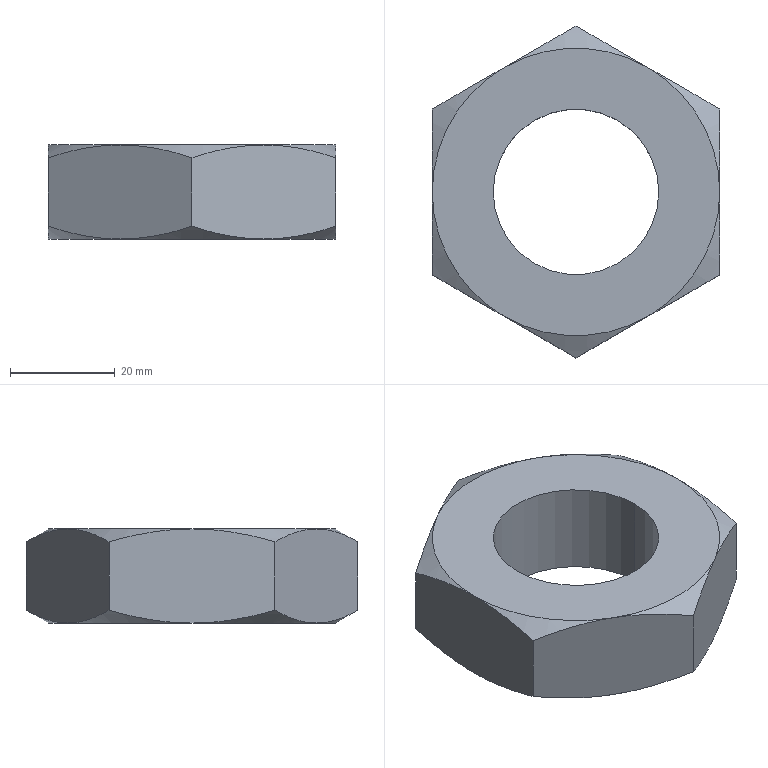Part | SolidWorks | features BaseBody 1 | 1 solid | 22 faces | box 55 x 63.509 x 18 mm | volume 32614 mm3 | cone 12 | plane 8 | cylinder 2 | commonest cylinder face diameters 31.67 x2
STEP:
#1=CARTESIAN_POINT('',(15.835,0.,18.));
#2=VERTEX_POINT('',#1);
#3=CARTESIAN_POINT('',(-15.835,0.,18.));
#4=VERTEX_POINT('',#3);
#5=CARTESIAN_POINT('',(0.,0.,18.));
#6=DIRECTION('',(0.,0.,-1.));
#7=DIRECTION('',(-1.,0.,0.));
#8=AXIS2_PLACEMENT_3D('',#5,#6,#7);
#9=CIRCLE('',#8,15.835);
#10=EDGE_CURVE('',#2,#4,#9,.T.);
#11=ORIENTED_EDGE('',*,*,#10,.F.);
#12=CARTESIAN_POINT('',(15.835,0.,0.));
#13=VERTEX_POINT('',#12);
#14=CARTESIAN_POINT('',(15.835,0.,18.));
#15=DIRECTION('',(0.,0.,-1.));
#16=VECTOR('',#15,1000.);
#17=LINE('',#14,#16);
#18=EDGE_CURVE('',#2,#13,#17,.T.);
#19=ORIENTED_EDGE('',*,*,#18,.T.);
#20=CARTESIAN_POINT('',(-15.835,0.,0.));
#21=VERTEX_POINT('',#20);
#22=CARTESIAN_POINT('',(0.,0.,0.));
#23=DIRECTION('',(0.,0.,-1.));
#24=DIRECTION('',(-1.,0.,0.));
#25=AXIS2_PLACEMENT_3D('',#22,#23,#24);
#26=CIRCLE('',#25,15.835);
#27=EDGE_CURVE('',#13,#21,#26,.T.);
#28=ORIENTED_EDGE('',*,*,#27,.T.);
#29=CARTESIAN_POINT('',(-15.835,0.,18.));
#30=DIRECTION('',(0.,0.,-1.));
#31=VECTOR('',#30,1000.);
#32=LINE('',#29,#31);
#33=EDGE_CURVE('',#4,#21,#32,.T.);
#34=ORIENTED_EDGE('',*,*,#33,.F.);
#35=EDGE_LOOP('',(#11,#19,#28,#34));
#36=FACE_OUTER_BOUND('',#35,.T.);
#37=CARTESIAN_POINT('',(0.,0.,18.));
#38=DIRECTION('',(0.,0.,-1.));
#39=DIRECTION('',(-1.,0.,0.));
#40=AXIS2_PLACEMENT_3D('',#37,#38,#39);
#41=CYLINDRICAL_SURFACE('',#40,15.835);
#42=ADVANCED_FACE('',(#36),#41,.F.);
#43=CARTESIAN_POINT('',(13.75,-23.816,0.));
#44=VERTEX_POINT('',#43);
#45=CARTESIAN_POINT('',(27.5,0.,0.));
#46=VERTEX_POINT('',#45);
#47=CARTESIAN_POINT('',(0.,0.,0.));
#48=DIRECTION('',(0.,0.,1.));
#49=DIRECTION('',(1.,0.,0.));
#50=AXIS2_PLACEMENT_3D('',#47,#48,#49);
#51=CIRCLE('',#50,27.5);
#52=EDGE_CURVE('',#44,#46,#51,.T.);
#53=ORIENTED_EDGE('',*,*,#52,.F.);
#54=CARTESIAN_POINT('',(-13.75,-23.816,0.));
#55=VERTEX_POINT('',#54);
#56=CARTESIAN_POINT('',(0.,0.,0.));
#57=DIRECTION('',(0.,0.,1.));
#58=DIRECTION('',(1.,0.,0.));
#59=AXIS2_PLACEMENT_3D('',#56,#57,#58);
#60=CIRCLE('',#59,27.5);
#61=EDGE_CURVE('',#55,#44,#60,.T.);
#62=ORIENTED_EDGE('',*,*,#61,.F.);
#63=CARTESIAN_POINT('',(-27.5,0.,0.));
#64=VERTEX_POINT('',#63);
#65=CARTESIAN_POINT('',(0.,0.,0.));
#66=DIRECTION('',(0.,0.,1.));
#67=DIRECTION('',(1.,0.,0.));
#68=AXIS2_PLACEMENT_3D('',#65,#66,#67);
#69=CIRCLE('',#68,27.5);
#70=EDGE_CURVE('',#64,#55,#69,.T.);
#71=ORIENTED_EDGE('',*,*,#70,.F.);
#72=CARTESIAN_POINT('',(-13.75,23.816,0.));
#73=VERTEX_POINT('',#72);
#74=CARTESIAN_POINT('',(0.,0.,0.));
#75=DIRECTION('',(0.,0.,1.));
#76=DIRECTION('',(0.,-1.,0.));
#77=AXIS2_PLACEMENT_3D('',#74,#75,#76);
#78=CIRCLE('',#77,27.5);
#79=EDGE_CURVE('',#73,#64,#78,.T.);
#80=ORIENTED_EDGE('',*,*,#79,.F.);
#81=CARTESIAN_POINT('',(13.75,23.816,0.));
#82=VERTEX_POINT('',#81);
#83=CARTESIAN_POINT('',(0.,0.,0.));
#84=DIRECTION('',(0.,0.,1.));
#85=DIRECTION('',(1.,0.,0.));
#86=AXIS2_PLACEMENT_3D('',#83,#84,#85);
#87=CIRCLE('',#86,27.5);
#88=EDGE_CURVE('',#82,#73,#87,.T.);
#89=ORIENTED_EDGE('',*,*,#88,.F.);
#90=CARTESIAN_POINT('',(0.,0.,0.));
#91=DIRECTION('',(0.,0.,1.));
#92=DIRECTION('',(1.,0.,0.));
#93=AXIS2_PLACEMENT_3D('',#90,#91,#92);
#94=CIRCLE('',#93,27.5);
#95=EDGE_CURVE('',#46,#82,#94,.T.);
#96=ORIENTED_EDGE('',*,*,#95,.F.);
#97=EDGE_LOOP('',(#53,#62,#71,#80,#89,#96));
#98=FACE_OUTER_BOUND('',#97,.T.);
#99=CARTESIAN_POINT('',(0.,0.,0.));
#100=DIRECTION('',(0.,0.,-1.));
#101=DIRECTION('',(-1.,0.,0.));
#102=AXIS2_PLACEMENT_3D('',#99,#100,#101);
#103=CIRCLE('',#102,15.835);
#104=EDGE_CURVE('',#21,#13,#103,.T.);
#105=ORIENTED_EDGE('',*,*,#104,.F.);
#106=ORIENTED_EDGE('',*,*,#27,.F.);
#107=EDGE_LOOP('',(#105,#106));
#108=FACE_BOUND('',#107,.T.);
#109=CARTESIAN_POINT('',(-27.5,47.631,0.));
#110=DIRECTION('',(0.,0.,1.));
#111=DIRECTION('',(1.,0.,0.));
#112=AXIS2_PLACEMENT_3D('',#109,#110,#111);
#113=PLANE('',#112);
#114=ADVANCED_FACE('',(#98,#108),#113,.F.);
#115=CARTESIAN_POINT('',(27.5,15.877,2.456));
#116=VERTEX_POINT('',#115);
#117=CARTESIAN_POINT('',(27.5,15.877,2.456));
#118=CARTESIAN_POINT('',(27.5,13.283,1.707));
#119=CARTESIAN_POINT('',(27.5,10.669,1.09));
#120=CARTESIAN_POINT('',(27.5,5.383,0.2348));
#121=CARTESIAN_POINT('',(27.5,2.71,0.));
#122=CARTESIAN_POINT('',(27.5,0.,0.));
#123=B_SPLINE_CURVE_WITH_KNOTS('',3,(#117,#118,#119,#120,#121,#122),.UNSPECIFIED.,.F.,.F.,(4,2,4),(0.,0.008033,0.01607),.UNSPECIFIED.);
#124=EDGE_CURVE('',#116,#46,#123,.T.);
#125=ORIENTED_EDGE('',*,*,#124,.T.);
#126=ORIENTED_EDGE('',*,*,#95,.T.);
#127=CARTESIAN_POINT('',(13.75,23.816,0.));
#128=CARTESIAN_POINT('',(16.097,22.461,0.));
#129=CARTESIAN_POINT('',(18.412,21.124,0.2348));
#130=CARTESIAN_POINT('',(22.99,18.481,1.09));
#131=CARTESIAN_POINT('',(25.254,17.174,1.707));
#132=CARTESIAN_POINT('',(27.5,15.877,2.456));
#133=B_SPLINE_CURVE_WITH_KNOTS('',3,(#127,#128,#129,#130,#131,#132),.UNSPECIFIED.,.F.,.F.,(4,2,4),(0.,0.008033,0.01607),.UNSPECIFIED.);
#134=EDGE_CURVE('',#82,#116,#133,.T.);
#135=ORIENTED_EDGE('',*,*,#134,.T.);
#136=EDGE_LOOP('',(#125,#126,#135));
#137=FACE_OUTER_BOUND('',#136,.T.);
#138=CARTESIAN_POINT('',(0.,0.,2.471));
#139=DIRECTION('',(0.,0.,1.));
#140=DIRECTION('',(1.,0.,0.));
#141=AXIS2_PLACEMENT_3D('',#138,#139,#140);
#142=CONICAL_SURFACE('',#141,31.78,1.047);
#143=ADVANCED_FACE('',(#137),#142,.T.);
#144=ORIENTED_EDGE('',*,*,#52,.T.);
#145=CARTESIAN_POINT('',(27.5,-15.877,2.456));
#146=VERTEX_POINT('',#145);
#147=CARTESIAN_POINT('',(27.5,0.,0.));
#148=CARTESIAN_POINT('',(27.5,-2.71,0.));
#149=CARTESIAN_POINT('',(27.5,-5.383,0.2348));
#150=CARTESIAN_POINT('',(27.5,-10.669,1.09));
#151=CARTESIAN_POINT('',(27.5,-13.283,1.707));
#152=CARTESIAN_POINT('',(27.5,-15.877,2.456));
#153=B_SPLINE_CURVE_WITH_KNOTS('',3,(#147,#148,#149,#150,#151,#152),.UNSPECIFIED.,.F.,.F.,(4,2,4),(0.,0.008033,0.01607),.UNSPECIFIED.);
#154=EDGE_CURVE('',#46,#146,#153,.T.);
#155=ORIENTED_EDGE('',*,*,#154,.T.);
#156=CARTESIAN_POINT('',(27.5,-15.877,2.456));
#157=CARTESIAN_POINT('',(25.254,-17.174,1.707));
#158=CARTESIAN_POINT('',(22.99,-18.481,1.09));
#159=CARTESIAN_POINT('',(18.412,-21.124,0.2348));
#160=CARTESIAN_POINT('',(16.097,-22.461,0.));
#161=CARTESIAN_POINT('',(13.75,-23.816,0.));
#162=B_SPLINE_CURVE_WITH_KNOTS('',3,(#156,#157,#158,#159,#160,#161),.UNSPECIFIED.,.F.,.F.,(4,2,4),(0.,0.008033,0.01607),.UNSPECIFIED.);
#163=EDGE_CURVE('',#146,#44,#162,.T.);
#164=ORIENTED_EDGE('',*,*,#163,.T.);
#165=EDGE_LOOP('',(#144,#155,#164));
#166=FACE_OUTER_BOUND('',#165,.T.);
#167=CARTESIAN_POINT('',(0.,0.,2.471));
#168=DIRECTION('',(0.,0.,1.));
#169=DIRECTION('',(1.,0.,0.));
#170=AXIS2_PLACEMENT_3D('',#167,#168,#169);
#171=CONICAL_SURFACE('',#170,31.78,1.047);
#172=ADVANCED_FACE('',(#166),#171,.T.);
#173=ORIENTED_EDGE('',*,*,#61,.T.);
#174=CARTESIAN_POINT('',(-0.000000014,-31.754,2.456));
#175=VERTEX_POINT('',#174);
#176=CARTESIAN_POINT('',(13.75,-23.816,0.));
#177=CARTESIAN_POINT('',(11.403,-25.17,0.));
#178=CARTESIAN_POINT('',(9.088,-26.507,0.2348));
#179=CARTESIAN_POINT('',(4.51,-29.15,1.09));
#180=CARTESIAN_POINT('',(2.246,-30.457,1.707));
#181=CARTESIAN_POINT('',(-0.000000014,-31.754,2.456));
#182=B_SPLINE_CURVE_WITH_KNOTS('',3,(#176,#177,#178,#179,#180,#181),.UNSPECIFIED.,.F.,.F.,(4,2,4),(0.,0.008033,0.01607),.UNSPECIFIED.);
#183=EDGE_CURVE('',#44,#175,#182,.T.);
#184=ORIENTED_EDGE('',*,*,#183,.T.);
#185=CARTESIAN_POINT('',(-0.000000014,-31.754,2.456));
#186=CARTESIAN_POINT('',(-2.246,-30.457,1.707));
#187=CARTESIAN_POINT('',(-4.51,-29.15,1.09));
#188=CARTESIAN_POINT('',(-9.088,-26.507,0.2348));
#189=CARTESIAN_POINT('',(-11.403,-25.17,0.));
#190=CARTESIAN_POINT('',(-13.75,-23.816,0.));
#191=B_SPLINE_CURVE_WITH_KNOTS('',3,(#185,#186,#187,#188,#189,#190),.UNSPECIFIED.,.F.,.F.,(4,2,4),(0.,0.008033,0.01607),.UNSPECIFIED.);
#192=EDGE_CURVE('',#175,#55,#191,.T.);
#193=ORIENTED_EDGE('',*,*,#192,.T.);
#194=EDGE_LOOP('',(#173,#184,#193));
#195=FACE_OUTER_BOUND('',#194,.T.);
#196=CARTESIAN_POINT('',(0.,0.,2.471));
#197=DIRECTION('',(0.,0.,1.));
#198=DIRECTION('',(1.,0.,0.));
#199=AXIS2_PLACEMENT_3D('',#196,#197,#198);
#200=CONICAL_SURFACE('',#199,31.78,1.047);
#201=ADVANCED_FACE('',(#195),#200,.T.);
#202=ORIENTED_EDGE('',*,*,#70,.T.);
#203=CARTESIAN_POINT('',(-27.5,-15.877,2.456));
#204=VERTEX_POINT('',#203);
#205=CARTESIAN_POINT('',(-13.75,-23.816,0.));
#206=CARTESIAN_POINT('',(-16.097,-22.461,0.));
#207=CARTESIAN_POINT('',(-18.412,-21.124,0.2348));
#208=CARTESIAN_POINT('',(-22.99,-18.481,1.09));
#209=CARTESIAN_POINT('',(-25.254,-17.174,1.707));
#210=CARTESIAN_POINT('',(-27.5,-15.877,2.456));
#211=B_SPLINE_CURVE_WITH_KNOTS('',3,(#205,#206,#207,#208,#209,#210),.UNSPECIFIED.,.F.,.F.,(4,2,4),(0.,0.008033,0.01607),.UNSPECIFIED.);
#212=EDGE_CURVE('',#55,#204,#211,.T.);
#213=ORIENTED_EDGE('',*,*,#212,.T.);
#214=CARTESIAN_POINT('',(-27.5,-15.877,2.456));
#215=CARTESIAN_POINT('',(-27.5,-13.283,1.707));
#216=CARTESIAN_POINT('',(-27.5,-10.669,1.09));
#217=CARTESIAN_POINT('',(-27.5,-5.383,0.2348));
#218=CARTESIAN_POINT('',(-27.5,-2.71,0.));
#219=CARTESIAN_POINT('',(-27.5,0.,0.));
#220=B_SPLINE_CURVE_WITH_KNOTS('',3,(#214,#215,#216,#217,#218,#219),.UNSPECIFIED.,.F.,.F.,(4,2,4),(0.,0.008033,0.01607),.UNSPECIFIED.);
#221=EDGE_CURVE('',#204,#64,#220,.T.);
#222=ORIENTED_EDGE('',*,*,#221,.T.);
#223=EDGE_LOOP('',(#202,#213,#222));
#224=FACE_OUTER_BOUND('',#223,.T.);
#225=CARTESIAN_POINT('',(0.,0.,2.471));
#226=DIRECTION('',(0.,0.,1.));
#227=DIRECTION('',(1.,0.,0.));
#228=AXIS2_PLACEMENT_3D('',#225,#226,#227);
#229=CONICAL_SURFACE('',#228,31.78,1.047);
#230=ADVANCED_FACE('',(#224),#229,.T.);
#231=CARTESIAN_POINT('',(-27.5,15.877,2.456));
#232=VERTEX_POINT('',#231);
#233=CARTESIAN_POINT('',(-27.5,15.877,2.456));
#234=CARTESIAN_POINT('',(-25.254,17.174,1.707));
#235=CARTESIAN_POINT('',(-22.99,18.481,1.09));
#236=CARTESIAN_POINT('',(-18.412,21.124,0.2348));
#237=CARTESIAN_POINT('',(-16.097,22.461,0.));
#238=CARTESIAN_POINT('',(-13.75,23.816,0.));
#239=B_SPLINE_CURVE_WITH_KNOTS('',3,(#233,#234,#235,#236,#237,#238),.UNSPECIFIED.,.F.,.F.,(4,2,4),(0.,0.008033,0.01607),.UNSPECIFIED.);
#240=EDGE_CURVE('',#232,#73,#239,.T.);
#241=ORIENTED_EDGE('',*,*,#240,.T.);
#242=ORIENTED_EDGE('',*,*,#79,.T.);
#243=CARTESIAN_POINT('',(-27.5,0.,0.));
#244=CARTESIAN_POINT('',(-27.5,2.71,0.));
#245=CARTESIAN_POINT('',(-27.5,5.383,0.2348));
#246=CARTESIAN_POINT('',(-27.5,10.669,1.09));
#247=CARTESIAN_POINT('',(-27.5,13.283,1.707));
#248=CARTESIAN_POINT('',(-27.5,15.877,2.456));
#249=B_SPLINE_CURVE_WITH_KNOTS('',3,(#243,#244,#245,#246,#247,#248),.UNSPECIFIED.,.F.,.F.,(4,2,4),(0.,0.008033,0.01607),.UNSPECIFIED.);
#250=EDGE_CURVE('',#64,#232,#249,.T.);
#251=ORIENTED_EDGE('',*,*,#250,.T.);
#252=EDGE_LOOP('',(#241,#242,#251));
#253=FACE_OUTER_BOUND('',#252,.T.);
#254=CARTESIAN_POINT('',(0.,0.,2.471));
#255=DIRECTION('',(0.,0.,1.));
#256=DIRECTION('',(0.,-1.,0.));
#257=AXIS2_PLACEMENT_3D('',#254,#255,#256);
#258=CONICAL_SURFACE('',#257,31.78,1.047);
#259=ADVANCED_FACE('',(#253),#258,.T.);
#260=CARTESIAN_POINT('',(-0.000000038,31.754,2.456));
#261=VERTEX_POINT('',#260);
#262=CARTESIAN_POINT('',(-0.000000038,31.754,2.456));
#263=CARTESIAN_POINT('',(2.246,30.457,1.707));
#264=CARTESIAN_POINT('',(4.51,29.15,1.09));
#265=CARTESIAN_POINT('',(9.088,26.507,0.2348));
#266=CARTESIAN_POINT('',(11.403,25.17,0.));
#267=CARTESIAN_POINT('',(13.75,23.816,0.));
#268=B_SPLINE_CURVE_WITH_KNOTS('',3,(#262,#263,#264,#265,#266,#267),.UNSPECIFIED.,.F.,.F.,(4,2,4),(0.,0.008033,0.01607),.UNSPECIFIED.);
#269=EDGE_CURVE('',#261,#82,#268,.T.);
#270=ORIENTED_EDGE('',*,*,#269,.T.);
#271=ORIENTED_EDGE('',*,*,#88,.T.);
#272=CARTESIAN_POINT('',(-13.75,23.816,0.));
#273=CARTESIAN_POINT('',(-11.403,25.17,0.));
#274=CARTESIAN_POINT('',(-9.088,26.507,0.2348));
#275=CARTESIAN_POINT('',(-4.51,29.15,1.09));
#276=CARTESIAN_POINT('',(-2.246,30.457,1.707));
#277=CARTESIAN_POINT('',(-0.000000038,31.754,2.456));
#278=B_SPLINE_CURVE_WITH_KNOTS('',3,(#272,#273,#274,#275,#276,#277),.UNSPECIFIED.,.F.,.F.,(4,2,4),(0.,0.008033,0.01607),.UNSPECIFIED.);
#279=EDGE_CURVE('',#73,#261,#278,.T.);
#280=ORIENTED_EDGE('',*,*,#279,.T.);
#281=EDGE_LOOP('',(#270,#271,#280));
#282=FACE_OUTER_BOUND('',#281,.T.);
#283=CARTESIAN_POINT('',(0.,0.,2.471));
#284=DIRECTION('',(0.,0.,1.));
#285=DIRECTION('',(1.,0.,0.));
#286=AXIS2_PLACEMENT_3D('',#283,#284,#285);
#287=CONICAL_SURFACE('',#286,31.78,1.047);
#288=ADVANCED_FACE('',(#282),#287,.T.);
#289=ORIENTED_EDGE('',*,*,#18,.F.);
#290=CARTESIAN_POINT('',(0.,0.,18.));
#291=DIRECTION('',(0.,0.,-1.));
#292=DIRECTION('',(-1.,0.,0.));
#293=AXIS2_PLACEMENT_3D('',#290,#291,#292);
#294=CIRCLE('',#293,15.835);
#295=EDGE_CURVE('',#4,#2,#294,.T.);
#296=ORIENTED_EDGE('',*,*,#295,.F.);
#297=ORIENTED_EDGE('',*,*,#33,.T.);
#298=ORIENTED_EDGE('',*,*,#104,.T.);
#299=EDGE_LOOP('',(#289,#296,#297,#298));
#300=FACE_OUTER_BOUND('',#299,.T.);
#301=CARTESIAN_POINT('',(0.,0.,18.));
#302=DIRECTION('',(0.,0.,-1.));
#303=DIRECTION('',(-1.,0.,0.));
#304=AXIS2_PLACEMENT_3D('',#301,#302,#303);
#305=CYLINDRICAL_SURFACE('',#304,15.835);
#306=ADVANCED_FACE('',(#300),#305,.F.);
#307=CARTESIAN_POINT('',(27.5,-15.877,15.544));
#308=VERTEX_POINT('',#307);
#309=CARTESIAN_POINT('',(27.5,-15.877,18.));
#310=DIRECTION('',(0.,0.,1.));
#311=VECTOR('',#310,1000.);
#312=LINE('',#309,#311);
#313=EDGE_CURVE('',#146,#308,#312,.T.);
#314=ORIENTED_EDGE('',*,*,#313,.F.);
#315=ORIENTED_EDGE('',*,*,#154,.F.);
#316=ORIENTED_EDGE('',*,*,#124,.F.);
#317=CARTESIAN_POINT('',(27.5,15.877,15.544));
#318=VERTEX_POINT('',#317);
#319=CARTESIAN_POINT('',(27.5,15.877,18.));
#320=DIRECTION('',(0.,0.,-1.));
#321=VECTOR('',#320,1000.);
#322=LINE('',#319,#321);
#323=EDGE_CURVE('',#318,#116,#322,.T.);
#324=ORIENTED_EDGE('',*,*,#323,.F.);
#325=CARTESIAN_POINT('',(27.5,0.,18.));
#326=VERTEX_POINT('',#325);
#327=CARTESIAN_POINT('',(27.5,0.,18.));
#328=CARTESIAN_POINT('',(27.5,2.71,18.));
#329=CARTESIAN_POINT('',(27.5,5.383,17.765));
#330=CARTESIAN_POINT('',(27.5,10.669,16.91));
#331=CARTESIAN_POINT('',(27.5,13.283,16.293));
#332=CARTESIAN_POINT('',(27.5,15.877,15.544));
#333=B_SPLINE_CURVE_WITH_KNOTS('',3,(#327,#328,#329,#330,#331,#332),.UNSPECIFIED.,.F.,.F.,(4,2,4),(0.,0.008033,0.01607),.UNSPECIFIED.);
#334=EDGE_CURVE('',#326,#318,#333,.T.);
#335=ORIENTED_EDGE('',*,*,#334,.F.);
#336=CARTESIAN_POINT('',(27.5,-15.877,15.544));
#337=CARTESIAN_POINT('',(27.5,-13.283,16.293));
#338=CARTESIAN_POINT('',(27.5,-10.669,16.91));
#339=CARTESIAN_POINT('',(27.5,-5.383,17.765));
#340=CARTESIAN_POINT('',(27.5,-2.71,18.));
#341=CARTESIAN_POINT('',(27.5,0.,18.));
#342=B_SPLINE_CURVE_WITH_KNOTS('',3,(#336,#337,#338,#339,#340,#341),.UNSPECIFIED.,.F.,.F.,(4,2,4),(0.,0.008033,0.01607),.UNSPECIFIED.);
#343=EDGE_CURVE('',#308,#326,#342,.T.);
#344=ORIENTED_EDGE('',*,*,#343,.F.);
#345=EDGE_LOOP('',(#314,#315,#316,#324,#335,#344));
#346=FACE_OUTER_BOUND('',#345,.T.);
#347=CARTESIAN_POINT('',(27.5,-15.877,18.));
#348=DIRECTION('',(-1.,0.,0.));
#349=DIRECTION('',(0.,-1.,0.));
#350=AXIS2_PLACEMENT_3D('',#347,#348,#349);
#351=PLANE('',#350);
#352=ADVANCED_FACE('',(#346),#351,.F.);
#353=ORIENTED_EDGE('',*,*,#323,.T.);
#354=ORIENTED_EDGE('',*,*,#134,.F.);
#355=ORIENTED_EDGE('',*,*,#269,.F.);
#356=CARTESIAN_POINT('',(0.,31.754,15.544));
#357=VERTEX_POINT('',#356);
#358=CARTESIAN_POINT('',(0.,31.754,18.));
#359=DIRECTION('',(0.,0.,-1.));
#360=VECTOR('',#359,1000.);
#361=LINE('',#358,#360);
#362=EDGE_CURVE('',#357,#261,#361,.T.);
#363=ORIENTED_EDGE('',*,*,#362,.F.);
#364=CARTESIAN_POINT('',(13.75,23.816,18.));
#365=VERTEX_POINT('',#364);
#366=CARTESIAN_POINT('',(13.75,23.816,18.));
#367=CARTESIAN_POINT('',(11.403,25.17,18.));
#368=CARTESIAN_POINT('',(9.088,26.507,17.765));
#369=CARTESIAN_POINT('',(4.51,29.15,16.91));
#370=CARTESIAN_POINT('',(2.246,30.457,16.293));
#371=CARTESIAN_POINT('',(0.,31.754,15.544));
#372=B_SPLINE_CURVE_WITH_KNOTS('',3,(#366,#367,#368,#369,#370,#371),.UNSPECIFIED.,.F.,.F.,(4,2,4),(0.,0.008033,0.01607),.UNSPECIFIED.);
#373=EDGE_CURVE('',#365,#357,#372,.T.);
#374=ORIENTED_EDGE('',*,*,#373,.F.);
#375=CARTESIAN_POINT('',(27.5,15.877,15.544));
#376=CARTESIAN_POINT('',(25.254,17.174,16.293));
#377=CARTESIAN_POINT('',(22.99,18.481,16.91));
#378=CARTESIAN_POINT('',(18.412,21.124,17.765));
#379=CARTESIAN_POINT('',(16.097,22.461,18.));
#380=CARTESIAN_POINT('',(13.75,23.816,18.));
#381=B_SPLINE_CURVE_WITH_KNOTS('',3,(#375,#376,#377,#378,#379,#380),.UNSPECIFIED.,.F.,.F.,(4,2,4),(0.,0.008033,0.01607),.UNSPECIFIED.);
#382=EDGE_CURVE('',#318,#365,#381,.T.);
#383=ORIENTED_EDGE('',*,*,#382,.F.);
#384=EDGE_LOOP('',(#353,#354,#355,#363,#374,#383));
#385=FACE_OUTER_BOUND('',#384,.T.);
#386=CARTESIAN_POINT('',(27.5,15.877,18.));
#387=DIRECTION('',(-0.5,-0.866,0.));
#388=DIRECTION('',(0.866,-0.5,0.));
#389=AXIS2_PLACEMENT_3D('',#386,#387,#388);
#390=PLANE('',#389);
#391=ADVANCED_FACE('',(#385),#390,.F.);
#392=CARTESIAN_POINT('',(-0.000000052,-31.754,15.544));
#393=VERTEX_POINT('',#392);
#394=CARTESIAN_POINT('',(0.,-31.754,18.));
#395=DIRECTION('',(0.,0.,1.));
#396=VECTOR('',#395,1000.);
#397=LINE('',#394,#396);
#398=EDGE_CURVE('',#175,#393,#397,.T.);
#399=ORIENTED_EDGE('',*,*,#398,.F.);
#400=ORIENTED_EDGE('',*,*,#183,.F.);
#401=ORIENTED_EDGE('',*,*,#163,.F.);
#402=ORIENTED_EDGE('',*,*,#313,.T.);
#403=CARTESIAN_POINT('',(13.75,-23.816,18.));
#404=VERTEX_POINT('',#403);
#405=CARTESIAN_POINT('',(13.75,-23.816,18.));
#406=CARTESIAN_POINT('',(16.097,-22.461,18.));
#407=CARTESIAN_POINT('',(18.412,-21.124,17.765));
#408=CARTESIAN_POINT('',(22.99,-18.481,16.91));
#409=CARTESIAN_POINT('',(25.254,-17.174,16.293));
#410=CARTESIAN_POINT('',(27.5,-15.877,15.544));
#411=B_SPLINE_CURVE_WITH_KNOTS('',3,(#405,#406,#407,#408,#409,#410),.UNSPECIFIED.,.F.,.F.,(4,2,4),(0.,0.008033,0.01607),.UNSPECIFIED.);
#412=EDGE_CURVE('',#404,#308,#411,.T.);
#413=ORIENTED_EDGE('',*,*,#412,.F.);
#414=CARTESIAN_POINT('',(-0.000000052,-31.754,15.544));
#415=CARTESIAN_POINT('',(2.246,-30.457,16.293));
#416=CARTESIAN_POINT('',(4.51,-29.15,16.91));
#417=CARTESIAN_POINT('',(9.088,-26.507,17.765));
#418=CARTESIAN_POINT('',(11.403,-25.17,18.));
#419=CARTESIAN_POINT('',(13.75,-23.816,18.));
#420=B_SPLINE_CURVE_WITH_KNOTS('',3,(#414,#415,#416,#417,#418,#419),.UNSPECIFIED.,.F.,.F.,(4,2,4),(0.,0.008033,0.01607),.UNSPECIFIED.);
#421=EDGE_CURVE('',#393,#404,#420,.T.);
#422=ORIENTED_EDGE('',*,*,#421,.F.);
#423=EDGE_LOOP('',(#399,#400,#401,#402,#413,#422));
#424=FACE_OUTER_BOUND('',#423,.T.);
#425=CARTESIAN_POINT('',(0.,-31.754,18.));
#426=DIRECTION('',(-0.5,0.866,0.));
#427=DIRECTION('',(-0.866,-0.5,0.));
#428=AXIS2_PLACEMENT_3D('',#425,#426,#427);
#429=PLANE('',#428);
#430=ADVANCED_FACE('',(#424),#429,.F.);
#431=CARTESIAN_POINT('',(-27.5,-15.877,15.544));
#432=VERTEX_POINT('',#431);
#433=CARTESIAN_POINT('',(-27.5,-15.877,18.));
#434=DIRECTION('',(0.,0.,1.));
#435=VECTOR('',#434,1000.);
#436=LINE('',#433,#435);
#437=EDGE_CURVE('',#204,#432,#436,.T.);
#438=ORIENTED_EDGE('',*,*,#437,.F.);
#439=ORIENTED_EDGE('',*,*,#212,.F.);
#440=ORIENTED_EDGE('',*,*,#192,.F.);
#441=ORIENTED_EDGE('',*,*,#398,.T.);
#442=CARTESIAN_POINT('',(-13.75,-23.816,18.));
#443=VERTEX_POINT('',#442);
#444=CARTESIAN_POINT('',(-13.75,-23.816,18.));
#445=CARTESIAN_POINT('',(-11.403,-25.17,18.));
#446=CARTESIAN_POINT('',(-9.088,-26.507,17.765));
#447=CARTESIAN_POINT('',(-4.51,-29.15,16.91));
#448=CARTESIAN_POINT('',(-2.246,-30.457,16.293));
#449=CARTESIAN_POINT('',(-0.000000052,-31.754,15.544));
#450=B_SPLINE_CURVE_WITH_KNOTS('',3,(#444,#445,#446,#447,#448,#449),.UNSPECIFIED.,.F.,.F.,(4,2,4),(0.,0.008033,0.01607),.UNSPECIFIED.);
#451=EDGE_CURVE('',#443,#393,#450,.T.);
#452=ORIENTED_EDGE('',*,*,#451,.F.);
#453=CARTESIAN_POINT('',(-27.5,-15.877,15.544));
#454=CARTESIAN_POINT('',(-25.254,-17.174,16.293));
#455=CARTESIAN_POINT('',(-22.99,-18.481,16.91));
#456=CARTESIAN_POINT('',(-18.412,-21.124,17.765));
#457=CARTESIAN_POINT('',(-16.097,-22.461,18.));
#458=CARTESIAN_POINT('',(-13.75,-23.816,18.));
#459=B_SPLINE_CURVE_WITH_KNOTS('',3,(#453,#454,#455,#456,#457,#458),.UNSPECIFIED.,.F.,.F.,(4,2,4),(0.,0.008033,0.01607),.UNSPECIFIED.);
#460=EDGE_CURVE('',#432,#443,#459,.T.);
#461=ORIENTED_EDGE('',*,*,#460,.F.);
#462=EDGE_LOOP('',(#438,#439,#440,#441,#452,#461));
#463=FACE_OUTER_BOUND('',#462,.T.);
#464=CARTESIAN_POINT('',(-27.5,-15.877,18.));
#465=DIRECTION('',(0.5,0.866,0.));
#466=DIRECTION('',(-0.866,0.5,0.));
#467=AXIS2_PLACEMENT_3D('',#464,#465,#466);
#468=PLANE('',#467);
#469=ADVANCED_FACE('',(#463),#468,.F.);
#470=CARTESIAN_POINT('',(-27.5,15.877,15.544));
#471=VERTEX_POINT('',#470);
#472=CARTESIAN_POINT('',(-27.5,15.877,18.));
#473=DIRECTION('',(0.,0.,1.));
#474=VECTOR('',#473,1000.);
#475=LINE('',#472,#474);
#476=EDGE_CURVE('',#232,#471,#475,.T.);
#477=ORIENTED_EDGE('',*,*,#476,.F.);
#478=ORIENTED_EDGE('',*,*,#250,.F.);
#479=ORIENTED_EDGE('',*,*,#221,.F.);
#480=ORIENTED_EDGE('',*,*,#437,.T.);
#481=CARTESIAN_POINT('',(-27.5,0.,18.));
#482=VERTEX_POINT('',#481);
#483=CARTESIAN_POINT('',(-27.5,0.,18.));
#484=CARTESIAN_POINT('',(-27.5,-2.71,18.));
#485=CARTESIAN_POINT('',(-27.5,-5.383,17.765));
#486=CARTESIAN_POINT('',(-27.5,-10.669,16.91));
#487=CARTESIAN_POINT('',(-27.5,-13.283,16.293));
#488=CARTESIAN_POINT('',(-27.5,-15.877,15.544));
#489=B_SPLINE_CURVE_WITH_KNOTS('',3,(#483,#484,#485,#486,#487,#488),.UNSPECIFIED.,.F.,.F.,(4,2,4),(0.,0.008033,0.01607),.UNSPECIFIED.);
#490=EDGE_CURVE('',#482,#432,#489,.T.);
#491=ORIENTED_EDGE('',*,*,#490,.F.);
#492=CARTESIAN_POINT('',(-27.5,15.877,15.544));
#493=CARTESIAN_POINT('',(-27.5,13.283,16.293));
#494=CARTESIAN_POINT('',(-27.5,10.669,16.91));
#495=CARTESIAN_POINT('',(-27.5,5.383,17.765));
#496=CARTESIAN_POINT('',(-27.5,2.71,18.));
#497=CARTESIAN_POINT('',(-27.5,0.,18.));
#498=B_SPLINE_CURVE_WITH_KNOTS('',3,(#492,#493,#494,#495,#496,#497),.UNSPECIFIED.,.F.,.F.,(4,2,4),(0.,0.008033,0.01607),.UNSPECIFIED.);
#499=EDGE_CURVE('',#471,#482,#498,.T.);
#500=ORIENTED_EDGE('',*,*,#499,.F.);
#501=EDGE_LOOP('',(#477,#478,#479,#480,#491,#500));
#502=FACE_OUTER_BOUND('',#501,.T.);
#503=CARTESIAN_POINT('',(-27.5,15.877,18.));
#504=DIRECTION('',(1.,0.,0.));
#505=DIRECTION('',(0.,1.,0.));
#506=AXIS2_PLACEMENT_3D('',#503,#504,#505);
#507=PLANE('',#506);
#508=ADVANCED_FACE('',(#502),#507,.F.);
#509=ORIENTED_EDGE('',*,*,#362,.T.);
#510=ORIENTED_EDGE('',*,*,#279,.F.);
#511=ORIENTED_EDGE('',*,*,#240,.F.);
#512=ORIENTED_EDGE('',*,*,#476,.T.);
#513=CARTESIAN_POINT('',(-13.75,23.816,18.));
#514=VERTEX_POINT('',#513);
#515=CARTESIAN_POINT('',(-13.75,23.816,18.));
#516=CARTESIAN_POINT('',(-16.097,22.461,18.));
#517=CARTESIAN_POINT('',(-18.412,21.124,17.765));
#518=CARTESIAN_POINT('',(-22.99,18.481,16.91));
#519=CARTESIAN_POINT('',(-25.254,17.174,16.293));
#520=CARTESIAN_POINT('',(-27.5,15.877,15.544));
#521=B_SPLINE_CURVE_WITH_KNOTS('',3,(#515,#516,#517,#518,#519,#520),.UNSPECIFIED.,.F.,.F.,(4,2,4),(0.,0.008033,0.01607),.UNSPECIFIED.);
#522=EDGE_CURVE('',#514,#471,#521,.T.);
#523=ORIENTED_EDGE('',*,*,#522,.F.);
#524=CARTESIAN_POINT('',(0.,31.754,15.544));
#525=CARTESIAN_POINT('',(-2.246,30.457,16.293));
#526=CARTESIAN_POINT('',(-4.51,29.15,16.91));
#527=CARTESIAN_POINT('',(-9.088,26.507,17.765));
#528=CARTESIAN_POINT('',(-11.403,25.17,18.));
#529=CARTESIAN_POINT('',(-13.75,23.816,18.));
#530=B_SPLINE_CURVE_WITH_KNOTS('',3,(#524,#525,#526,#527,#528,#529),.UNSPECIFIED.,.F.,.F.,(4,2,4),(0.,0.008033,0.01607),.UNSPECIFIED.);
#531=EDGE_CURVE('',#357,#514,#530,.T.);
#532=ORIENTED_EDGE('',*,*,#531,.F.);
#533=EDGE_LOOP('',(#509,#510,#511,#512,#523,#532));
#534=FACE_OUTER_BOUND('',#533,.T.);
#535=CARTESIAN_POINT('',(0.,31.754,18.));
#536=DIRECTION('',(0.5,-0.866,0.));
#537=DIRECTION('',(0.866,0.5,0.));
#538=AXIS2_PLACEMENT_3D('',#535,#536,#537);
#539=PLANE('',#538);
#540=ADVANCED_FACE('',(#534),#539,.F.);
#541=CARTESIAN_POINT('',(0.,0.,18.));
#542=DIRECTION('',(0.,0.,1.));
#543=DIRECTION('',(-1.,0.,0.));
#544=AXIS2_PLACEMENT_3D('',#541,#542,#543);
#545=CIRCLE('',#544,27.5);
#546=EDGE_CURVE('',#482,#443,#545,.T.);
#547=ORIENTED_EDGE('',*,*,#546,.T.);
#548=CARTESIAN_POINT('',(0.,0.,18.));
#549=DIRECTION('',(0.,0.,1.));
#550=DIRECTION('',(-1.,0.,0.));
#551=AXIS2_PLACEMENT_3D('',#548,#549,#550);
#552=CIRCLE('',#551,27.5);
#553=EDGE_CURVE('',#443,#404,#552,.T.);
#554=ORIENTED_EDGE('',*,*,#553,.T.);
#555=CARTESIAN_POINT('',(0.,0.,18.));
#556=DIRECTION('',(0.,0.,1.));
#557=DIRECTION('',(0.,1.,0.));
#558=AXIS2_PLACEMENT_3D('',#555,#556,#557);
#559=CIRCLE('',#558,27.5);
#560=EDGE_CURVE('',#404,#326,#559,.T.);
#561=ORIENTED_EDGE('',*,*,#560,.T.);
#562=CARTESIAN_POINT('',(0.,0.,18.));
#563=DIRECTION('',(0.,0.,1.));
#564=DIRECTION('',(-1.,0.,0.));
#565=AXIS2_PLACEMENT_3D('',#562,#563,#564);
#566=CIRCLE('',#565,27.5);
#567=EDGE_CURVE('',#326,#365,#566,.T.);
#568=ORIENTED_EDGE('',*,*,#567,.T.);
#569=CARTESIAN_POINT('',(0.,0.,18.));
#570=DIRECTION('',(0.,0.,1.));
#571=DIRECTION('',(-1.,0.,0.));
#572=AXIS2_PLACEMENT_3D('',#569,#570,#571);
#573=CIRCLE('',#572,27.5);
#574=EDGE_CURVE('',#365,#514,#573,.T.);
#575=ORIENTED_EDGE('',*,*,#574,.T.);
#576=CARTESIAN_POINT('',(0.,0.,18.));
#577=DIRECTION('',(0.,0.,1.));
#578=DIRECTION('',(0.,1.,0.));
#579=AXIS2_PLACEMENT_3D('',#576,#577,#578);
#580=CIRCLE('',#579,27.5);
#581=EDGE_CURVE('',#514,#482,#580,.T.);
#582=ORIENTED_EDGE('',*,*,#581,.T.);
#583=EDGE_LOOP('',(#547,#554,#561,#568,#575,#582));
#584=FACE_OUTER_BOUND('',#583,.T.);
#585=ORIENTED_EDGE('',*,*,#295,.T.);
#586=ORIENTED_EDGE('',*,*,#10,.T.);
#587=EDGE_LOOP('',(#585,#586));
#588=FACE_BOUND('',#587,.T.);
#589=CARTESIAN_POINT('',(-27.5,47.631,18.));
#590=DIRECTION('',(0.,0.,1.));
#591=DIRECTION('',(1.,0.,0.));
#592=AXIS2_PLACEMENT_3D('',#589,#590,#591);
#593=PLANE('',#592);
#594=ADVANCED_FACE('',(#584,#588),#593,.T.);
#595=ORIENTED_EDGE('',*,*,#343,.T.);
#596=ORIENTED_EDGE('',*,*,#560,.F.);
#597=ORIENTED_EDGE('',*,*,#412,.T.);
#598=EDGE_LOOP('',(#595,#596,#597));
#599=FACE_OUTER_BOUND('',#598,.T.);
#600=CARTESIAN_POINT('',(0.,0.,15.529));
#601=DIRECTION('',(0.,0.,-1.));
#602=DIRECTION('',(0.,1.,0.));
#603=AXIS2_PLACEMENT_3D('',#600,#601,#602);
#604=CONICAL_SURFACE('',#603,31.78,1.047);
#605=ADVANCED_FACE('',(#599),#604,.T.);
#606=ORIENTED_EDGE('',*,*,#567,.F.);
#607=ORIENTED_EDGE('',*,*,#334,.T.);
#608=ORIENTED_EDGE('',*,*,#382,.T.);
#609=EDGE_LOOP('',(#606,#607,#608));
#610=FACE_OUTER_BOUND('',#609,.T.);
#611=CARTESIAN_POINT('',(0.,0.,15.529));
#612=DIRECTION('',(0.,0.,-1.));
#613=DIRECTION('',(-1.,0.,0.));
#614=AXIS2_PLACEMENT_3D('',#611,#612,#613);
#615=CONICAL_SURFACE('',#614,31.78,1.047);
#616=ADVANCED_FACE('',(#610),#615,.T.);
#617=ORIENTED_EDGE('',*,*,#531,.T.);
#618=ORIENTED_EDGE('',*,*,#574,.F.);
#619=ORIENTED_EDGE('',*,*,#373,.T.);
#620=EDGE_LOOP('',(#617,#618,#619));
#621=FACE_OUTER_BOUND('',#620,.T.);
#622=CARTESIAN_POINT('',(0.,0.,15.529));
#623=DIRECTION('',(0.,0.,-1.));
#624=DIRECTION('',(-1.,0.,0.));
#625=AXIS2_PLACEMENT_3D('',#622,#623,#624);
#626=CONICAL_SURFACE('',#625,31.78,1.047);
#627=ADVANCED_FACE('',(#621),#626,.T.);
#628=ORIENTED_EDGE('',*,*,#421,.T.);
#629=ORIENTED_EDGE('',*,*,#553,.F.);
#630=ORIENTED_EDGE('',*,*,#451,.T.);
#631=EDGE_LOOP('',(#628,#629,#630));
#632=FACE_OUTER_BOUND('',#631,.T.);
#633=CARTESIAN_POINT('',(0.,0.,15.529));
#634=DIRECTION('',(0.,0.,-1.));
#635=DIRECTION('',(-1.,0.,0.));
#636=AXIS2_PLACEMENT_3D('',#633,#634,#635);
#637=CONICAL_SURFACE('',#636,31.78,1.047);
#638=ADVANCED_FACE('',(#632),#637,.T.);
#639=ORIENTED_EDGE('',*,*,#460,.T.);
#640=ORIENTED_EDGE('',*,*,#546,.F.);
#641=ORIENTED_EDGE('',*,*,#490,.T.);
#642=EDGE_LOOP('',(#639,#640,#641));
#643=FACE_OUTER_BOUND('',#642,.T.);
#644=CARTESIAN_POINT('',(0.,0.,15.529));
#645=DIRECTION('',(0.,0.,-1.));
#646=DIRECTION('',(-1.,0.,0.));
#647=AXIS2_PLACEMENT_3D('',#644,#645,#646);
#648=CONICAL_SURFACE('',#647,31.78,1.047);
#649=ADVANCED_FACE('',(#643),#648,.T.);
#650=ORIENTED_EDGE('',*,*,#499,.T.);
#651=ORIENTED_EDGE('',*,*,#581,.F.);
#652=ORIENTED_EDGE('',*,*,#522,.T.);
#653=EDGE_LOOP('',(#650,#651,#652));
#654=FACE_OUTER_BOUND('',#653,.T.);
#655=CARTESIAN_POINT('',(0.,0.,15.529));
#656=DIRECTION('',(0.,0.,-1.));
#657=DIRECTION('',(0.,1.,0.));
#658=AXIS2_PLACEMENT_3D('',#655,#656,#657);
#659=CONICAL_SURFACE('',#658,31.78,1.047);
#660=ADVANCED_FACE('',(#654),#659,.T.);
#661=CLOSED_SHELL('',(#42,#114,#143,#172,#201,#230,#259,#288,#306,#352,#391,#430,#469,#508,#540,#594,#605,#616,#627,#638,#649,#660));
#662=MANIFOLD_SOLID_BREP('',#661);
#663=CARTESIAN_POINT('',(0.,0.,0.));
#664=DIRECTION('',(0.,0.,1.));
#665=DIRECTION('',(1.,0.,0.));
#666=AXIS2_PLACEMENT_3D('',#663,#664,#665);
#667=(LENGTH_UNIT()NAMED_UNIT(*)SI_UNIT(.MILLI.,.METRE.));
#668=UNCERTAINTY_MEASURE_WITH_UNIT(LENGTH_MEASURE(0.00001),#667,'','');
#669=(NAMED_UNIT(*)PLANE_ANGLE_UNIT()SI_UNIT($,.RADIAN.));
#670=(NAMED_UNIT(*)SI_UNIT($,.STERADIAN.)SOLID_ANGLE_UNIT());
#671=(GEOMETRIC_REPRESENTATION_CONTEXT(3)GLOBAL_UNCERTAINTY_ASSIGNED_CONTEXT((#668))GLOBAL_UNIT_ASSIGNED_CONTEXT((#667,#669,#670))REPRESENTATION_CONTEXT('',''));
#672=ADVANCED_BREP_SHAPE_REPRESENTATION('',(#662,#666),#671);